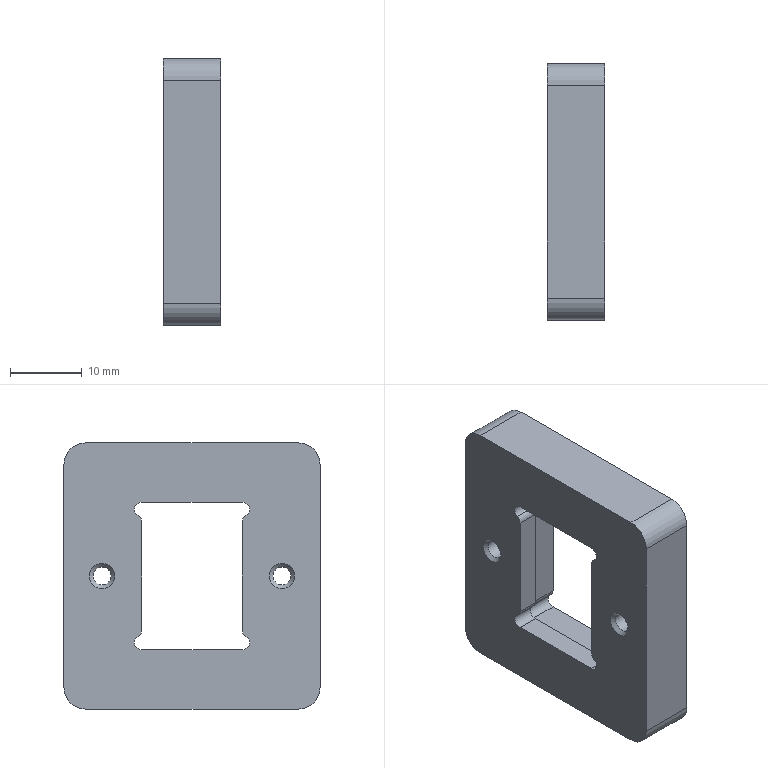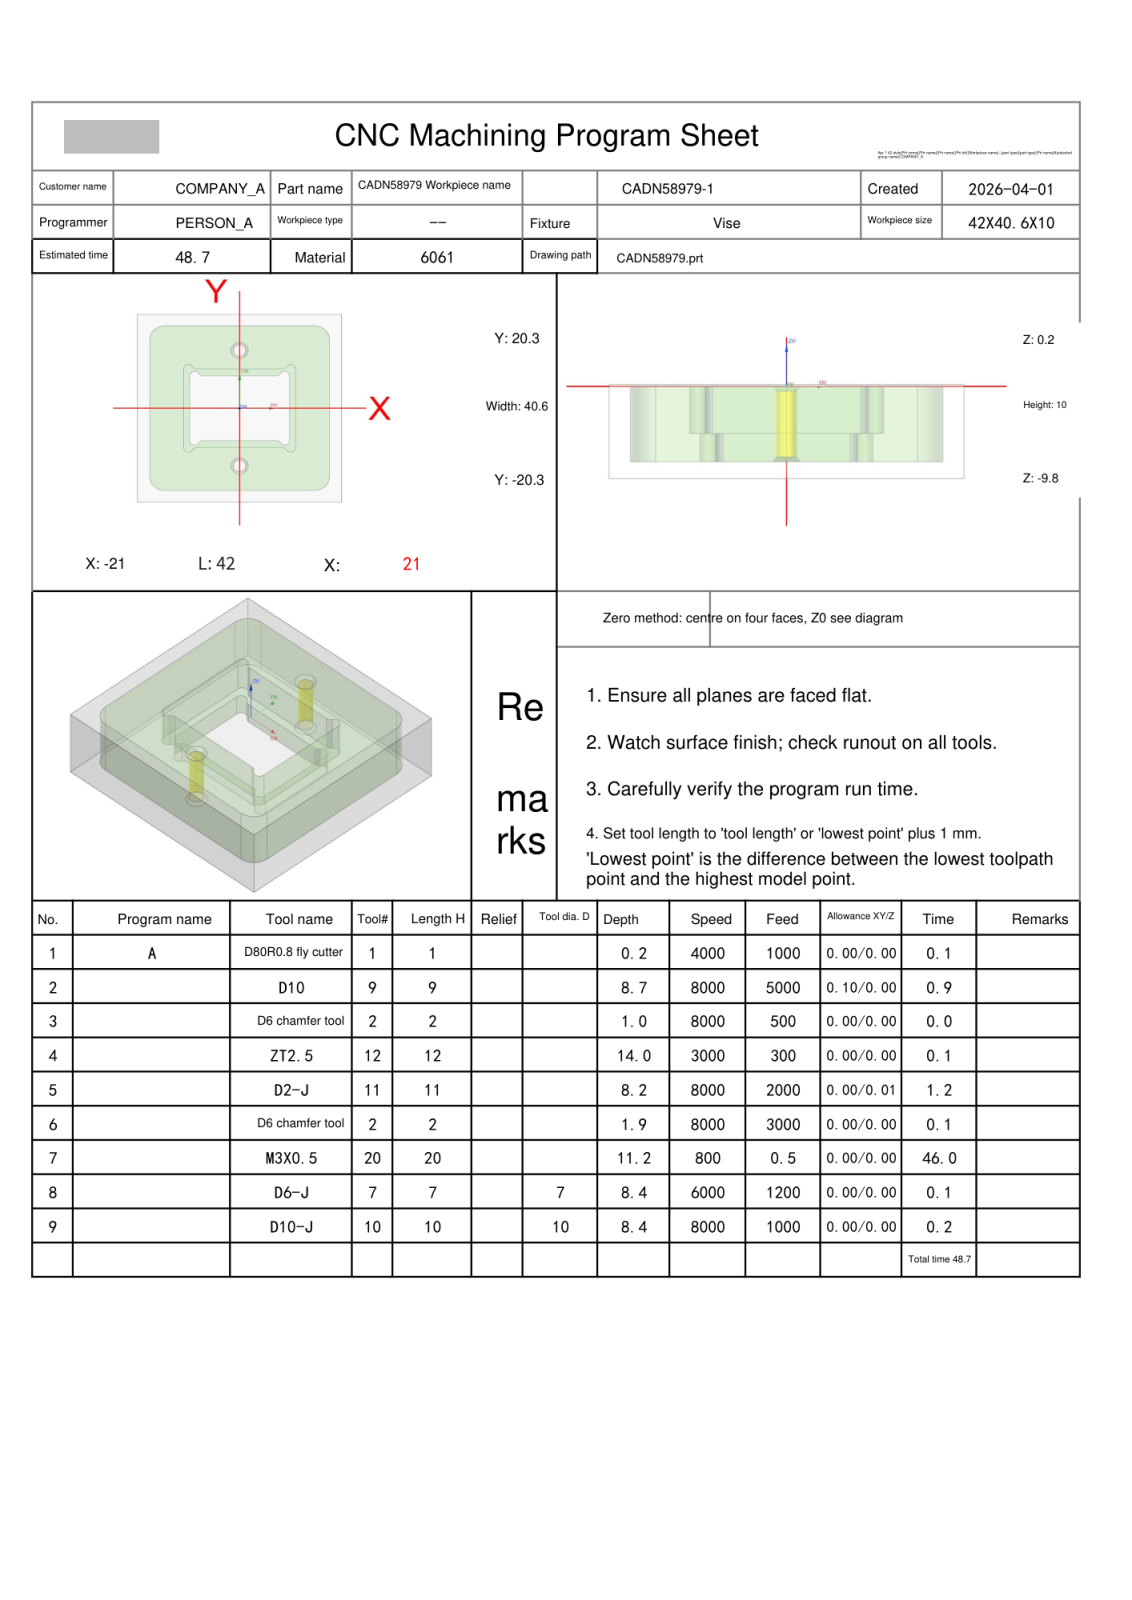NC program | NX | posted by the shop | part box 8 x 35.6 x 37 mm
Lines 315 to 1416 of 3954:
N5 T11 M06
(D2-J  D=2. R=0. H=11 ce=0.00 di=0.01)
G00 G90 G54 X-9.75 Y-2.651 M03 S8000
G43 H11 Z20.
M08
Z.55
G01 X-9.76 Y-2.653 Z.436 F1600.
X-9.786 Y-2.659 Z.333
X-9.828 Y-2.671 Z.242
X-9.882 Y-2.688 Z.161
X-9.944 Y-2.712 Z.089
X-10.014 Y-2.742 Z.027
X-10.088 Y-2.779 Z-.026
X-10.162 Y-2.824 Z-.071
X-10.236 Y-2.877 Z-.109
X-10.306 Y-2.939 Z-.139
X-10.368 Y-3.011 Z-.162
X-10.422 Y-3.092 Z-.179
X-10.464 Y-3.184 Z-.191
X-10.49 Y-3.286 Z-.198
X-10.5 Y-3.401 Z-.2
Y-8.5 F2000.
G02 X-8.768 Y-7.5 I1.732 J-1.
G01 X-6.401
X-6.387 Y-7.484
X-6.398 Y-7.439 Z-.202
X-6.432 Y-7.368 Z-.205
X-6.488 Y-7.273 Z-.209
X-6.707 Y-6.956 Z-.222
X-6.93 Y-6.661 Z-.234
X-7.229 Y-6.288 Z-.25
X-7.746 Y-5.698 Z-.276
X-8.213 Y-5.213 Z-.3
X-8.698 Y-4.746 Z-.323
X-9.288 Y-4.229 Z-.35
X-9.661 Y-3.93 Z-.366
X-9.956 Y-3.707 Z-.378
X-10.273 Y-3.488 Z-.391
X-10.368 Y-3.432 Z-.394
X-10.439 Y-3.398 Z-.397
X-10.484 Y-3.387 Z-.399
X-10.5 Y-3.401 Z-.4
Y-8.5
G02 X-8.768 Y-7.5 I1.732 J-1.
G01 X-6.401
X-6.387 Y-7.484
X-6.398 Y-7.439 Z-.402
X-6.432 Y-7.368 Z-.405
X-6.488 Y-7.273 Z-.409
X-6.707 Y-6.956 Z-.421
X-6.93 Y-6.661 Z-.434
X-7.229 Y-6.288 Z-.45
X-7.746 Y-5.698 Z-.476
X-8.213 Y-5.213 Z-.5
X-8.698 Y-4.746 Z-.523
X-9.288 Y-4.229 Z-.549
X-9.661 Y-3.93 Z-.565
X-9.956 Y-3.707 Z-.578
X-10.273 Y-3.488 Z-.59
X-10.368 Y-3.432 Z-.594
X-10.439 Y-3.398 Z-.597
X-10.484 Y-3.387 Z-.599
X-10.5 Y-3.401
Y-8.5
G02 X-8.768 Y-7.5 I1.732 J-1.
G01 X-6.401
X-6.387 Y-7.484 Z-.6
X-6.398 Y-7.439 Z-.602
X-6.432 Y-7.368 Z-.605
X-6.488 Y-7.273 Z-.608
X-6.707 Y-6.956 Z-.621
X-6.93 Y-6.661 Z-.633
X-7.229 Y-6.288 Z-.649
X-7.746 Y-5.698 Z-.676
X-8.213 Y-5.213 Z-.699
X-8.698 Y-4.746 Z-.723
X-9.288 Y-4.229 Z-.749
X-9.661 Y-3.93 Z-.765
X-9.956 Y-3.707 Z-.777
X-10.273 Y-3.488 Z-.79
X-10.368 Y-3.432 Z-.794
X-10.439 Y-3.398 Z-.797
X-10.484 Y-3.387 Z-.799
X-10.5 Y-3.401
Y-8.5
G02 X-8.768 Y-7.5 I1.732 J-1.
G01 X-6.401
X-6.387 Y-7.484 Z-.8
X-6.398 Y-7.439 Z-.802
X-6.432 Y-7.368 Z-.804
X-6.488 Y-7.273 Z-.808
X-6.707 Y-6.956 Z-.821
X-6.93 Y-6.661 Z-.833
X-7.229 Y-6.288 Z-.849
X-7.746 Y-5.698 Z-.876
X-8.213 Y-5.213 Z-.899
X-8.698 Y-4.746 Z-.922
X-9.288 Y-4.229 Z-.949
X-9.661 Y-3.93 Z-.965
X-9.956 Y-3.707 Z-.977
X-10.273 Y-3.488 Z-.99
X-10.368 Y-3.432 Z-.994
X-10.439 Y-3.398 Z-.997
X-10.484 Y-3.387 Z-.998
X-10.5 Y-3.401 Z-.999
Y-8.5
G02 X-8.768 Y-7.5 I1.732 J-1.
G01 X-6.401
X-6.387 Y-7.484 Z-1.
X-6.398 Y-7.439 Z-1.001
X-6.432 Y-7.368 Z-1.004
X-6.488 Y-7.273 Z-1.008
X-6.707 Y-6.956 Z-1.021
X-6.93 Y-6.661 Z-1.033
X-7.229 Y-6.288 Z-1.049
X-7.746 Y-5.698 Z-1.076
X-8.213 Y-5.213 Z-1.099
X-8.698 Y-4.746 Z-1.122
X-9.288 Y-4.229 Z-1.149
X-9.661 Y-3.93 Z-1.165
X-9.956 Y-3.707 Z-1.177
X-10.273 Y-3.488 Z-1.19
X-10.368 Y-3.432 Z-1.194
X-10.439 Y-3.398 Z-1.196
X-10.484 Y-3.387 Z-1.198
X-10.5 Y-3.401 Z-1.199
Y-8.5
G02 X-8.768 Y-7.5 I1.732 J-1.
G01 X-6.401
X-6.387 Y-7.484
X-6.398 Y-7.439 Z-1.201
X-6.432 Y-7.368 Z-1.204
X-6.488 Y-7.273 Z-1.208
X-6.707 Y-6.956 Z-1.221
X-6.93 Y-6.661 Z-1.233
X-7.229 Y-6.288 Z-1.249
X-7.746 Y-5.698 Z-1.275
X-8.213 Y-5.213 Z-1.299
X-8.698 Y-4.746 Z-1.322
X-9.288 Y-4.229 Z-1.349
X-9.661 Y-3.93 Z-1.365
X-9.956 Y-3.707 Z-1.377
X-10.273 Y-3.488 Z-1.39
X-10.368 Y-3.432 Z-1.393
X-10.439 Y-3.398 Z-1.396
X-10.484 Y-3.387 Z-1.398
X-10.5 Y-3.401 Z-1.399
Y-8.5
G02 X-8.768 Y-7.5 I1.732 J-1.
G01 X-6.401
X-6.387 Y-7.484
X-6.398 Y-7.439 Z-1.401
X-6.432 Y-7.368 Z-1.404
X-6.488 Y-7.273 Z-1.408
X-6.707 Y-6.956 Z-1.42
X-6.93 Y-6.661 Z-1.433
X-7.229 Y-6.288 Z-1.449
X-7.746 Y-5.698 Z-1.475
X-8.213 Y-5.213 Z-1.499
X-8.698 Y-4.746 Z-1.522
X-9.288 Y-4.229 Z-1.548
X-9.661 Y-3.93 Z-1.564
X-9.956 Y-3.707 Z-1.577
X-10.273 Y-3.488 Z-1.589
X-10.368 Y-3.432 Z-1.593
X-10.439 Y-3.398 Z-1.596
X-10.484 Y-3.387 Z-1.598
X-10.5 Y-3.401
Y-8.5
G02 X-8.768 Y-7.5 I1.732 J-1.
G01 X-6.401
X-6.387 Y-7.484 Z-1.599
X-6.398 Y-7.439 Z-1.601
X-6.432 Y-7.368 Z-1.604
X-6.488 Y-7.273 Z-1.607
X-6.707 Y-6.956 Z-1.62
X-6.93 Y-6.661 Z-1.632
X-7.229 Y-6.288 Z-1.648
X-7.746 Y-5.698 Z-1.675
X-8.213 Y-5.213 Z-1.698
X-8.698 Y-4.746 Z-1.722
X-9.288 Y-4.229 Z-1.748
X-9.661 Y-3.93 Z-1.764
X-9.956 Y-3.707 Z-1.776
X-10.273 Y-3.488 Z-1.789
X-10.368 Y-3.432 Z-1.793
X-10.439 Y-3.398 Z-1.796
X-10.484 Y-3.387 Z-1.798
X-10.5 Y-3.401
Y-8.5
G02 X-8.768 Y-7.5 I1.732 J-1.
G01 X-6.401
X-6.387 Y-7.484 Z-1.799
X-6.398 Y-7.439 Z-1.801
X-6.432 Y-7.368 Z-1.803
X-6.488 Y-7.273 Z-1.807
X-6.707 Y-6.956 Z-1.82
X-6.93 Y-6.661 Z-1.832
X-7.229 Y-6.288 Z-1.848
X-7.746 Y-5.698 Z-1.875
X-8.213 Y-5.213 Z-1.898
X-8.698 Y-4.746 Z-1.921
X-9.288 Y-4.229 Z-1.948
X-9.661 Y-3.93 Z-1.964
X-9.956 Y-3.707 Z-1.976
X-10.273 Y-3.488 Z-1.989
X-10.368 Y-3.432 Z-1.993
X-10.439 Y-3.398 Z-1.996
X-10.484 Y-3.387 Z-1.997
X-10.5 Y-3.401 Z-1.998
Y-8.5
G02 X-8.768 Y-7.5 I1.732 J-1.
G01 X-6.401
X-6.387 Y-7.484 Z-1.999
X-6.398 Y-7.439 Z-2.
X-6.432 Y-7.368 Z-2.003
X-6.488 Y-7.273 Z-2.007
X-6.707 Y-6.956 Z-2.02
X-6.93 Y-6.661 Z-2.032
X-7.229 Y-6.288 Z-2.048
X-7.746 Y-5.698 Z-2.075
X-8.213 Y-5.213 Z-2.098
X-8.698 Y-4.746 Z-2.121
X-9.288 Y-4.229 Z-2.148
X-9.661 Y-3.93 Z-2.164
X-9.956 Y-3.707 Z-2.176
X-10.273 Y-3.488 Z-2.189
X-10.368 Y-3.432 Z-2.193
X-10.439 Y-3.398 Z-2.195
X-10.484 Y-3.387 Z-2.197
X-10.5 Y-3.401 Z-2.198
Y-8.5
G02 X-8.768 Y-7.5 I1.732 J-1.
G01 X-6.401
X-6.387 Y-7.484
X-6.398 Y-7.439 Z-2.2
X-6.432 Y-7.368 Z-2.203
X-6.488 Y-7.273 Z-2.207
X-6.707 Y-6.956 Z-2.22
X-6.93 Y-6.661 Z-2.232
X-7.229 Y-6.288 Z-2.248
X-7.746 Y-5.698 Z-2.274
X-8.213 Y-5.213 Z-2.298
X-8.698 Y-4.746 Z-2.321
X-9.288 Y-4.229 Z-2.348
X-9.661 Y-3.93 Z-2.364
X-9.956 Y-3.707 Z-2.376
X-10.273 Y-3.488 Z-2.389
X-10.368 Y-3.432 Z-2.392
X-10.439 Y-3.398 Z-2.395
X-10.484 Y-3.387 Z-2.397
X-10.5 Y-3.401 Z-2.398
Y-8.5
G02 X-8.768 Y-7.5 I1.732 J-1.
G01 X-6.401
X-6.387 Y-7.484
X-6.398 Y-7.439 Z-2.4
X-6.432 Y-7.368 Z-2.403
X-6.488 Y-7.273 Z-2.407
X-6.707 Y-6.956 Z-2.419
X-6.93 Y-6.661 Z-2.432
X-7.229 Y-6.288 Z-2.448
X-7.746 Y-5.698 Z-2.474
X-8.213 Y-5.213 Z-2.498
X-8.698 Y-4.746 Z-2.521
X-9.288 Y-4.229 Z-2.547
X-9.661 Y-3.93 Z-2.563
X-9.956 Y-3.707 Z-2.576
X-10.273 Y-3.488 Z-2.588
X-10.368 Y-3.432 Z-2.592
X-10.439 Y-3.398 Z-2.595
X-10.484 Y-3.387 Z-2.597
X-10.5 Y-3.401
Y-8.5
G02 X-8.768 Y-7.5 I1.732 J-1.
G01 X-6.401
X-6.387 Y-7.484 Z-2.598
X-6.398 Y-7.439 Z-2.6
X-6.432 Y-7.368 Z-2.603
X-6.488 Y-7.273 Z-2.606
X-6.707 Y-6.956 Z-2.619
X-6.93 Y-6.661 Z-2.631
X-7.229 Y-6.288 Z-2.647
X-7.746 Y-5.698 Z-2.674
X-8.213 Y-5.213 Z-2.697
X-8.698 Y-4.746 Z-2.721
X-9.288 Y-4.229 Z-2.747
X-9.661 Y-3.93 Z-2.763
X-9.956 Y-3.707 Z-2.775
X-10.273 Y-3.488 Z-2.788
X-10.368 Y-3.432 Z-2.792
X-10.439 Y-3.398 Z-2.795
X-10.484 Y-3.387 Z-2.797
X-10.5 Y-3.401
Y-8.5
G02 X-8.768 Y-7.5 I1.732 J-1.
G01 X-6.401
X-6.387 Y-7.484 Z-2.798
X-6.398 Y-7.439 Z-2.8
X-6.432 Y-7.368 Z-2.802
X-6.488 Y-7.273 Z-2.806
X-6.707 Y-6.956 Z-2.819
X-6.93 Y-6.661 Z-2.831
X-7.229 Y-6.288 Z-2.847
X-7.746 Y-5.698 Z-2.874
X-8.213 Y-5.213 Z-2.897
X-8.698 Y-4.746 Z-2.92
X-9.288 Y-4.229 Z-2.947
X-9.661 Y-3.93 Z-2.963
X-9.956 Y-3.707 Z-2.975
X-10.273 Y-3.488 Z-2.988
X-10.368 Y-3.432 Z-2.992
X-10.439 Y-3.398 Z-2.995
X-10.484 Y-3.387 Z-2.996
X-10.5 Y-3.401 Z-2.997
Y-8.5
G02 X-8.768 Y-7.5 I1.732 J-1.
G01 X-6.401
X-6.387 Y-7.484 Z-2.998
X-6.398 Y-7.439 Z-2.999
X-6.432 Y-7.368 Z-3.002
X-6.488 Y-7.273 Z-3.006
X-6.707 Y-6.956 Z-3.019
X-6.93 Y-6.661 Z-3.031
X-7.229 Y-6.288 Z-3.047
X-7.746 Y-5.698 Z-3.074
X-8.213 Y-5.213 Z-3.097
X-8.698 Y-4.746 Z-3.12
X-9.288 Y-4.229 Z-3.147
X-9.661 Y-3.93 Z-3.163
X-9.956 Y-3.707 Z-3.175
X-10.273 Y-3.488 Z-3.188
X-10.368 Y-3.432 Z-3.192
X-10.439 Y-3.398 Z-3.194
X-10.484 Y-3.387 Z-3.196
X-10.5 Y-3.401 Z-3.197
Y-8.5
G02 X-8.768 Y-7.5 I1.732 J-1.
G01 X-6.401
X-6.387 Y-7.484
X-6.398 Y-7.439 Z-3.199
X-6.432 Y-7.368 Z-3.202
X-6.488 Y-7.273 Z-3.206
X-6.707 Y-6.956 Z-3.219
X-6.93 Y-6.661 Z-3.231
X-7.229 Y-6.288 Z-3.247
X-7.746 Y-5.698 Z-3.273
X-8.213 Y-5.213 Z-3.297
X-8.698 Y-4.746 Z-3.32
X-9.288 Y-4.229 Z-3.347
X-9.661 Y-3.93 Z-3.363
X-9.956 Y-3.707 Z-3.375
X-10.273 Y-3.488 Z-3.388
X-10.368 Y-3.432 Z-3.391
X-10.439 Y-3.398 Z-3.394
X-10.484 Y-3.387 Z-3.396
X-10.5 Y-3.401 Z-3.397
Y-8.5
G02 X-8.768 Y-7.5 I1.732 J-1.
G01 X-6.401
X-6.387 Y-7.484
X-6.398 Y-7.439 Z-3.399
X-6.432 Y-7.368 Z-3.402
X-6.488 Y-7.273 Z-3.406
X-6.707 Y-6.956 Z-3.418
X-6.93 Y-6.661 Z-3.431
X-7.229 Y-6.288 Z-3.447
X-7.746 Y-5.698 Z-3.473
X-8.213 Y-5.213 Z-3.497
X-8.698 Y-4.746 Z-3.52
X-9.288 Y-4.229 Z-3.546
X-9.661 Y-3.93 Z-3.562
X-9.956 Y-3.707 Z-3.575
X-10.273 Y-3.488 Z-3.587
X-10.368 Y-3.432 Z-3.591
X-10.439 Y-3.398 Z-3.594
X-10.484 Y-3.387 Z-3.596
X-10.5 Y-3.401
Y-8.5
G02 X-8.768 Y-7.5 I1.732 J-1.
G01 X-6.401
X-6.387 Y-7.484 Z-3.597
X-6.398 Y-7.439 Z-3.599
X-6.432 Y-7.368 Z-3.602
X-6.488 Y-7.273 Z-3.605
X-6.707 Y-6.956 Z-3.618
X-6.93 Y-6.661 Z-3.63
X-7.229 Y-6.288 Z-3.646
X-7.746 Y-5.698 Z-3.673
X-8.213 Y-5.213 Z-3.696
X-8.698 Y-4.746 Z-3.72
X-9.288 Y-4.229 Z-3.746
X-9.661 Y-3.93 Z-3.762
X-9.956 Y-3.707 Z-3.774
X-10.273 Y-3.488 Z-3.787
X-10.368 Y-3.432 Z-3.791
X-10.439 Y-3.398 Z-3.794
X-10.484 Y-3.387 Z-3.796
X-10.5 Y-3.401
Y-8.5
G02 X-8.768 Y-7.5 I1.732 J-1.
G01 X-6.401
X-6.387 Y-7.484 Z-3.797
X-6.398 Y-7.439 Z-3.799
X-6.432 Y-7.368 Z-3.801
X-6.488 Y-7.273 Z-3.805
X-6.707 Y-6.956 Z-3.818
X-6.93 Y-6.661 Z-3.83
X-7.229 Y-6.288 Z-3.846
X-7.746 Y-5.698 Z-3.873
X-8.213 Y-5.213 Z-3.896
X-8.698 Y-4.746 Z-3.919
X-9.288 Y-4.229 Z-3.946
X-9.661 Y-3.93 Z-3.962
X-9.956 Y-3.707 Z-3.974
X-10.273 Y-3.488 Z-3.987
X-10.368 Y-3.432 Z-3.991
X-10.439 Y-3.398 Z-3.994
X-10.484 Y-3.387 Z-3.995
X-10.5 Y-3.401 Z-3.996
Y-8.5
G02 X-8.768 Y-7.5 I1.732 J-1.
G01 X-6.401
X-6.387 Y-7.484 Z-3.997
X-6.398 Y-7.439 Z-3.998
X-6.432 Y-7.368 Z-4.001
X-6.488 Y-7.273 Z-4.005
X-6.707 Y-6.956 Z-4.018
X-6.93 Y-6.661 Z-4.03
X-7.229 Y-6.288 Z-4.046
X-7.746 Y-5.698 Z-4.073
X-8.213 Y-5.213 Z-4.096
X-8.698 Y-4.746 Z-4.119
X-9.288 Y-4.229 Z-4.146
X-9.661 Y-3.93 Z-4.162
X-9.956 Y-3.707 Z-4.174
X-10.273 Y-3.488 Z-4.187
X-10.368 Y-3.432 Z-4.191
X-10.439 Y-3.398 Z-4.193
X-10.484 Y-3.387 Z-4.195
X-10.5 Y-3.401 Z-4.196
Y-8.5
G02 X-8.768 Y-7.5 I1.732 J-1.
G01 X-6.401
X-6.387 Y-7.484
X-6.398 Y-7.439 Z-4.198
X-6.432 Y-7.368 Z-4.201
X-6.488 Y-7.273 Z-4.205
X-6.707 Y-6.956 Z-4.218
X-6.93 Y-6.661 Z-4.23
X-7.229 Y-6.288 Z-4.246
X-7.746 Y-5.698 Z-4.272
X-8.213 Y-5.213 Z-4.296
X-8.698 Y-4.746 Z-4.319
X-9.288 Y-4.229 Z-4.346
X-9.661 Y-3.93 Z-4.362
X-9.956 Y-3.707 Z-4.374
X-10.273 Y-3.488 Z-4.387
X-10.368 Y-3.432 Z-4.39
X-10.439 Y-3.398 Z-4.393
X-10.484 Y-3.387 Z-4.395
X-10.5 Y-3.401 Z-4.396
Y-8.5
G02 X-8.768 Y-7.5 I1.732 J-1.
G01 X-6.401
X-6.387 Y-7.484
X-6.398 Y-7.439 Z-4.398
X-6.432 Y-7.368 Z-4.401
X-6.488 Y-7.273 Z-4.405
X-6.707 Y-6.956 Z-4.417
X-6.93 Y-6.661 Z-4.43
X-7.229 Y-6.288 Z-4.446
X-7.746 Y-5.698 Z-4.472
X-8.213 Y-5.213 Z-4.496
X-8.698 Y-4.746 Z-4.519
X-9.288 Y-4.229 Z-4.545
X-9.661 Y-3.93 Z-4.561
X-9.956 Y-3.707 Z-4.574
X-10.273 Y-3.488 Z-4.586
X-10.368 Y-3.432 Z-4.59
X-10.439 Y-3.398 Z-4.593
X-10.484 Y-3.387 Z-4.595
X-10.5 Y-3.401
Y-8.5
G02 X-8.768 Y-7.5 I1.732 J-1.
G01 X-6.401
X-6.387 Y-7.484 Z-4.596
X-6.398 Y-7.439 Z-4.598
X-6.432 Y-7.368 Z-4.601
X-6.488 Y-7.273 Z-4.604
X-6.707 Y-6.956 Z-4.617
X-6.93 Y-6.661 Z-4.629
X-7.229 Y-6.288 Z-4.645
X-7.746 Y-5.698 Z-4.672
X-8.213 Y-5.213 Z-4.695
X-8.698 Y-4.746 Z-4.719
X-9.288 Y-4.229 Z-4.745
X-9.661 Y-3.93 Z-4.761
X-9.956 Y-3.707 Z-4.773
X-10.273 Y-3.488 Z-4.786
X-10.368 Y-3.432 Z-4.79
X-10.439 Y-3.398 Z-4.793
X-10.484 Y-3.387 Z-4.795
X-10.5 Y-3.401
Y-8.5
G02 X-8.768 Y-7.5 I1.732 J-1.
G01 X-6.401
X-6.387 Y-7.484 Z-4.796
X-6.398 Y-7.439 Z-4.798
X-6.432 Y-7.368 Z-4.8
X-6.488 Y-7.273 Z-4.804
X-6.707 Y-6.956 Z-4.817
X-6.93 Y-6.661 Z-4.829
X-7.229 Y-6.288 Z-4.845
X-7.746 Y-5.698 Z-4.872
X-8.213 Y-5.213 Z-4.895
X-8.698 Y-4.746 Z-4.918
X-9.288 Y-4.229 Z-4.945
X-9.661 Y-3.93 Z-4.961
X-9.956 Y-3.707 Z-4.973
X-10.273 Y-3.488 Z-4.986
X-10.368 Y-3.432 Z-4.99
X-10.439 Y-3.398 Z-4.993
X-10.484 Y-3.387 Z-4.994
X-10.5 Y-3.401 Z-4.995
Y-8.5
G02 X-8.768 Y-7.5 I1.732 J-1.
G01 X-6.401
X-6.286 Y-7.49 Z-4.993
X-6.184 Y-7.464 Z-4.986
X-6.092 Y-7.422 Z-4.975
X-6.011 Y-7.368 Z-4.957
X-5.939 Y-7.306 Z-4.934
X-5.877 Y-7.236 Z-4.904
X-5.824 Y-7.162 Z-4.867
X-5.779 Y-7.088 Z-4.821
X-5.742 Y-7.014 Z-4.768
X-5.712 Y-6.944 Z-4.706
X-5.688 Y-6.882 Z-4.635
X-5.671 Y-6.828 Z-4.553
X-5.659 Y-6.786 Z-4.462
X-5.653 Y-6.76 Z-4.359
X-5.651 Y-6.75 Z-4.245
G00 Z3.
X5.651
Z.55
G01 X5.653 Y-6.76 Z.436 F1600.
X5.659 Y-6.786 Z.333
X5.671 Y-6.828 Z.242
X5.688 Y-6.882 Z.161
X5.712 Y-6.944 Z.089
X5.742 Y-7.014 Z.027
X5.779 Y-7.088 Z-.026
X5.824 Y-7.162 Z-.071
X5.877 Y-7.236 Z-.109
X5.939 Y-7.306 Z-.139
X6.011 Y-7.368 Z-.162
X6.092 Y-7.422 Z-.179
X6.184 Y-7.464 Z-.191
X6.286 Y-7.49 Z-.198
X6.401 Y-7.5 Z-.2
X8.768 F2000.
G02 X10.5 Y-8.5 I0.0 J-2.
G01 Y-3.401
X10.484 Y-3.387
X10.439 Y-3.398 Z-.202
X10.368 Y-3.432 Z-.205
X10.273 Y-3.488 Z-.209
X9.956 Y-3.707 Z-.222
X9.661 Y-3.93 Z-.234
X9.288 Y-4.229 Z-.25
X8.698 Y-4.746 Z-.276
X8.213 Y-5.213 Z-.3
X7.746 Y-5.698 Z-.323
X7.229 Y-6.288 Z-.35
X6.93 Y-6.661 Z-.366
X6.707 Y-6.956 Z-.378
X6.488 Y-7.273 Z-.391
X6.432 Y-7.368 Z-.394
X6.398 Y-7.439 Z-.397
X6.387 Y-7.484 Z-.399
X6.401 Y-7.5 Z-.4
X8.768
G02 X10.5 Y-8.5 I0.0 J-2.
G01 Y-3.401
X10.484 Y-3.387
X10.439 Y-3.398 Z-.402
X10.368 Y-3.432 Z-.405
X10.273 Y-3.488 Z-.409
X9.956 Y-3.707 Z-.421
X9.661 Y-3.93 Z-.434
X9.288 Y-4.229 Z-.45
X8.698 Y-4.746 Z-.476
X8.213 Y-5.213 Z-.5
X7.746 Y-5.698 Z-.523
X7.229 Y-6.288 Z-.549
X6.93 Y-6.661 Z-.565
X6.707 Y-6.956 Z-.578
X6.488 Y-7.273 Z-.59
X6.432 Y-7.368 Z-.594
X6.398 Y-7.439 Z-.597
X6.387 Y-7.484 Z-.599
X6.401 Y-7.5
X8.768
G02 X10.5 Y-8.5 I0.0 J-2.
G01 Y-3.401
X10.484 Y-3.387 Z-.6
X10.439 Y-3.398 Z-.602
X10.368 Y-3.432 Z-.605
X10.273 Y-3.488 Z-.608
X9.956 Y-3.707 Z-.621
X9.661 Y-3.93 Z-.633
X9.288 Y-4.229 Z-.649
X8.698 Y-4.746 Z-.676
X8.213 Y-5.213 Z-.699
X7.746 Y-5.698 Z-.723
X7.229 Y-6.288 Z-.749
X6.93 Y-6.661 Z-.765
X6.707 Y-6.956 Z-.777
X6.488 Y-7.273 Z-.79
X6.432 Y-7.368 Z-.794
X6.398 Y-7.439 Z-.797
X6.387 Y-7.484 Z-.799
X6.401 Y-7.5
X8.768
G02 X10.5 Y-8.5 I0.0 J-2.
G01 Y-3.401
X10.484 Y-3.387 Z-.8
X10.439 Y-3.398 Z-.802
X10.368 Y-3.432 Z-.804
X10.273 Y-3.488 Z-.808
X9.956 Y-3.707 Z-.821
X9.661 Y-3.93 Z-.833
X9.288 Y-4.229 Z-.849
X8.698 Y-4.746 Z-.876
X8.213 Y-5.213 Z-.899
X7.746 Y-5.698 Z-.922
X7.229 Y-6.288 Z-.949
X6.93 Y-6.661 Z-.965
X6.707 Y-6.956 Z-.977
X6.488 Y-7.273 Z-.99
X6.432 Y-7.368 Z-.994
X6.398 Y-7.439 Z-.997
X6.387 Y-7.484 Z-.998
X6.401 Y-7.5 Z-.999
X8.768
G02 X10.5 Y-8.5 I0.0 J-2.
G01 Y-3.401
X10.484 Y-3.387 Z-1.
X10.439 Y-3.398 Z-1.001
X10.368 Y-3.432 Z-1.004
X10.273 Y-3.488 Z-1.008
X9.956 Y-3.707 Z-1.021
X9.661 Y-3.93 Z-1.033
X9.288 Y-4.229 Z-1.049
X8.698 Y-4.746 Z-1.076
X8.213 Y-5.213 Z-1.099
X7.746 Y-5.698 Z-1.122
X7.229 Y-6.288 Z-1.149
X6.93 Y-6.661 Z-1.165
X6.707 Y-6.956 Z-1.177
X6.488 Y-7.273 Z-1.19
X6.432 Y-7.368 Z-1.194
X6.398 Y-7.439 Z-1.196
X6.387 Y-7.484 Z-1.198
X6.401 Y-7.5 Z-1.199
X8.768
G02 X10.5 Y-8.5 I0.0 J-2.
G01 Y-3.401
X10.484 Y-3.387
X10.439 Y-3.398 Z-1.201
X10.368 Y-3.432 Z-1.204
X10.273 Y-3.488 Z-1.208
X9.956 Y-3.707 Z-1.221
X9.661 Y-3.93 Z-1.233
X9.288 Y-4.229 Z-1.249
X8.698 Y-4.746 Z-1.275
X8.213 Y-5.213 Z-1.299
X7.746 Y-5.698 Z-1.322
X7.229 Y-6.288 Z-1.349
X6.93 Y-6.661 Z-1.365
X6.707 Y-6.956 Z-1.377
X6.488 Y-7.273 Z-1.39
X6.432 Y-7.368 Z-1.393
X6.398 Y-7.439 Z-1.396
X6.387 Y-7.484 Z-1.398
X6.401 Y-7.5 Z-1.399
X8.768
G02 X10.5 Y-8.5 I0.0 J-2.
G01 Y-3.401
X10.484 Y-3.387
X10.439 Y-3.398 Z-1.401
X10.368 Y-3.432 Z-1.404
X10.273 Y-3.488 Z-1.408
X9.956 Y-3.707 Z-1.42
X9.661 Y-3.93 Z-1.433
X9.288 Y-4.229 Z-1.449
X8.698 Y-4.746 Z-1.475
X8.213 Y-5.213 Z-1.499
X7.746 Y-5.698 Z-1.522
X7.229 Y-6.288 Z-1.548
X6.93 Y-6.661 Z-1.564
X6.707 Y-6.956 Z-1.577
X6.488 Y-7.273 Z-1.589
X6.432 Y-7.368 Z-1.593
X6.398 Y-7.439 Z-1.596
X6.387 Y-7.484 Z-1.598
X6.401 Y-7.5
X8.768
G02 X10.5 Y-8.5 I0.0 J-2.
G01 Y-3.401
X10.484 Y-3.387 Z-1.599
X10.439 Y-3.398 Z-1.601
X10.368 Y-3.432 Z-1.604
X10.273 Y-3.488 Z-1.607
X9.956 Y-3.707 Z-1.62
X9.661 Y-3.93 Z-1.632
X9.288 Y-4.229 Z-1.648
X8.698 Y-4.746 Z-1.675
X8.213 Y-5.213 Z-1.698
X7.746 Y-5.698 Z-1.722
X7.229 Y-6.288 Z-1.748
X6.93 Y-6.661 Z-1.764
X6.707 Y-6.956 Z-1.776
X6.488 Y-7.273 Z-1.789
X6.432 Y-7.368 Z-1.793
X6.398 Y-7.439 Z-1.796
X6.387 Y-7.484 Z-1.798
X6.401 Y-7.5
X8.768
G02 X10.5 Y-8.5 I0.0 J-2.
G01 Y-3.401
X10.484 Y-3.387 Z-1.799
X10.439 Y-3.398 Z-1.801
X10.368 Y-3.432 Z-1.803
X10.273 Y-3.488 Z-1.807
X9.956 Y-3.707 Z-1.82
X9.661 Y-3.93 Z-1.832
X9.288 Y-4.229 Z-1.848
X8.698 Y-4.746 Z-1.875
X8.213 Y-5.213 Z-1.898
X7.746 Y-5.698 Z-1.921
X7.229 Y-6.288 Z-1.948
X6.93 Y-6.661 Z-1.964
X6.707 Y-6.956 Z-1.976
X6.488 Y-7.273 Z-1.989
X6.432 Y-7.368 Z-1.993
X6.398 Y-7.439 Z-1.996
X6.387 Y-7.484 Z-1.997
X6.401 Y-7.5 Z-1.998
X8.768
G02 X10.5 Y-8.5 I0.0 J-2.
G01 Y-3.401
X10.484 Y-3.387 Z-1.999
X10.439 Y-3.398 Z-2.
X10.368 Y-3.432 Z-2.003
X10.273 Y-3.488 Z-2.007
X9.956 Y-3.707 Z-2.02
X9.661 Y-3.93 Z-2.032
X9.288 Y-4.229 Z-2.048
X8.698 Y-4.746 Z-2.075
X8.213 Y-5.213 Z-2.098
X7.746 Y-5.698 Z-2.121
X7.229 Y-6.288 Z-2.148
X6.93 Y-6.661 Z-2.164
X6.707 Y-6.956 Z-2.176
X6.488 Y-7.273 Z-2.189
X6.432 Y-7.368 Z-2.193
X6.398 Y-7.439 Z-2.195
X6.387 Y-7.484 Z-2.197
X6.401 Y-7.5 Z-2.198
X8.768
G02 X10.5 Y-8.5 I0.0 J-2.
G01 Y-3.401
X10.484 Y-3.387
X10.439 Y-3.398 Z-2.2
X10.368 Y-3.432 Z-2.203
X10.273 Y-3.488 Z-2.207
X9.956 Y-3.707 Z-2.22
X9.661 Y-3.93 Z-2.232
X9.288 Y-4.229 Z-2.248
X8.698 Y-4.746 Z-2.274
X8.213 Y-5.213 Z-2.298
X7.746 Y-5.698 Z-2.321
X7.229 Y-6.288 Z-2.348
X6.93 Y-6.661 Z-2.364
X6.707 Y-6.956 Z-2.376
X6.488 Y-7.273 Z-2.389
X6.432 Y-7.368 Z-2.392
X6.398 Y-7.439 Z-2.395
X6.387 Y-7.484 Z-2.397
X6.401 Y-7.5 Z-2.398
X8.768
G02 X10.5 Y-8.5 I0.0 J-2.
G01 Y-3.401
X10.484 Y-3.387
X10.439 Y-3.398 Z-2.4
X10.368 Y-3.432 Z-2.403
X10.273 Y-3.488 Z-2.407
X9.956 Y-3.707 Z-2.419
X9.661 Y-3.93 Z-2.432
X9.288 Y-4.229 Z-2.448
X8.698 Y-4.746 Z-2.474
X8.213 Y-5.213 Z-2.498
X7.746 Y-5.698 Z-2.521
X7.229 Y-6.288 Z-2.547
X6.93 Y-6.661 Z-2.563
X6.707 Y-6.956 Z-2.576
X6.488 Y-7.273 Z-2.588
X6.432 Y-7.368 Z-2.592
X6.398 Y-7.439 Z-2.595
X6.387 Y-7.484 Z-2.597
X6.401 Y-7.5
X8.768
G02 X10.5 Y-8.5 I0.0 J-2.
G01 Y-3.401
X10.484 Y-3.387 Z-2.598
X10.439 Y-3.398 Z-2.6
X10.368 Y-3.432 Z-2.603
X10.273 Y-3.488 Z-2.606
X9.956 Y-3.707 Z-2.619
X9.661 Y-3.93 Z-2.631
X9.288 Y-4.229 Z-2.647
X8.698 Y-4.746 Z-2.674
X8.213 Y-5.213 Z-2.697
X7.746 Y-5.698 Z-2.721
X7.229 Y-6.288 Z-2.747
X6.93 Y-6.661 Z-2.763
X6.707 Y-6.956 Z-2.775
X6.488 Y-7.273 Z-2.788
X6.432 Y-7.368 Z-2.792
X6.398 Y-7.439 Z-2.795
X6.387 Y-7.484 Z-2.797
X6.401 Y-7.5
X8.768
G02 X10.5 Y-8.5 I0.0 J-2.
G01 Y-3.401
X10.484 Y-3.387 Z-2.798
X10.439 Y-3.398 Z-2.8
X10.368 Y-3.432 Z-2.802
X10.273 Y-3.488 Z-2.806
X9.956 Y-3.707 Z-2.819
X9.661 Y-3.93 Z-2.831
X9.288 Y-4.229 Z-2.847
X8.698 Y-4.746 Z-2.874
X8.213 Y-5.213 Z-2.897
X7.746 Y-5.698 Z-2.92
X7.229 Y-6.288 Z-2.947
X6.93 Y-6.661 Z-2.963
X6.707 Y-6.956 Z-2.975
X6.488 Y-7.273 Z-2.988
X6.432 Y-7.368 Z-2.992
X6.398 Y-7.439 Z-2.995
X6.387 Y-7.484 Z-2.996
X6.401 Y-7.5 Z-2.997
X8.768
G02 X10.5 Y-8.5 I0.0 J-2.
G01 Y-3.401
X10.484 Y-3.387 Z-2.998
X10.439 Y-3.398 Z-2.999
X10.368 Y-3.432 Z-3.002
X10.273 Y-3.488 Z-3.006
X9.956 Y-3.707 Z-3.019
X9.661 Y-3.93 Z-3.031
X9.288 Y-4.229 Z-3.047
X8.698 Y-4.746 Z-3.074
X8.213 Y-5.213 Z-3.097
X7.746 Y-5.698 Z-3.12
X7.229 Y-6.288 Z-3.147
X6.93 Y-6.661 Z-3.163
X6.707 Y-6.956 Z-3.175
X6.488 Y-7.273 Z-3.188
X6.432 Y-7.368 Z-3.192
X6.398 Y-7.439 Z-3.194
X6.387 Y-7.484 Z-3.196
X6.401 Y-7.5 Z-3.197
X8.768
G02 X10.5 Y-8.5 I0.0 J-2.
G01 Y-3.401
X10.484 Y-3.387
X10.439 Y-3.398 Z-3.199
X10.368 Y-3.432 Z-3.202
X10.273 Y-3.488 Z-3.206
X9.956 Y-3.707 Z-3.219
X9.661 Y-3.93 Z-3.231
X9.288 Y-4.229 Z-3.247
X8.698 Y-4.746 Z-3.273
X8.213 Y-5.213 Z-3.297
X7.746 Y-5.698 Z-3.32
X7.229 Y-6.288 Z-3.347
X6.93 Y-6.661 Z-3.363
X6.707 Y-6.956 Z-3.375
X6.488 Y-7.273 Z-3.388
X6.432 Y-7.368 Z-3.391
X6.398 Y-7.439 Z-3.394
X6.387 Y-7.484 Z-3.396
X6.401 Y-7.5 Z-3.397
X8.768
G02 X10.5 Y-8.5 I0.0 J-2.
G01 Y-3.401
X10.484 Y-3.387
X10.439 Y-3.398 Z-3.399
X10.368 Y-3.432 Z-3.402
X10.273 Y-3.488 Z-3.406
X9.956 Y-3.707 Z-3.418
X9.661 Y-3.93 Z-3.431
X9.288 Y-4.229 Z-3.447
X8.698 Y-4.746 Z-3.473
X8.213 Y-5.213 Z-3.497
X7.746 Y-5.698 Z-3.52
X7.229 Y-6.288 Z-3.546
X6.93 Y-6.661 Z-3.562
X6.707 Y-6.956 Z-3.575
X6.488 Y-7.273 Z-3.587
X6.432 Y-7.368 Z-3.591
X6.398 Y-7.439 Z-3.594
X6.387 Y-7.484 Z-3.596
X6.401 Y-7.5
X8.768
G02 X10.5 Y-8.5 I0.0 J-2.
G01 Y-3.401
X10.484 Y-3.387 Z-3.597
X10.439 Y-3.398 Z-3.599
X10.368 Y-3.432 Z-3.602
X10.273 Y-3.488 Z-3.605
X9.956 Y-3.707 Z-3.618
X9.661 Y-3.93 Z-3.63
X9.288 Y-4.229 Z-3.646
X8.698 Y-4.746 Z-3.673
X8.213 Y-5.213 Z-3.696
X7.746 Y-5.698 Z-3.72
X7.229 Y-6.288 Z-3.746
X6.93 Y-6.661 Z-3.762
X6.707 Y-6.956 Z-3.774
X6.488 Y-7.273 Z-3.787
X6.432 Y-7.368 Z-3.791
X6.398 Y-7.439 Z-3.794
X6.387 Y-7.484 Z-3.796
X6.401 Y-7.5
X8.768
G02 X10.5 Y-8.5 I0.0 J-2.
G01 Y-3.401
X10.484 Y-3.387 Z-3.797
X10.439 Y-3.398 Z-3.799
X10.368 Y-3.432 Z-3.801
X10.273 Y-3.488 Z-3.805
X9.956 Y-3.707 Z-3.818
X9.661 Y-3.93 Z-3.83
X9.288 Y-4.229 Z-3.846
X8.698 Y-4.746 Z-3.873
X8.213 Y-5.213 Z-3.896
X7.746 Y-5.698 Z-3.919
X7.229 Y-6.288 Z-3.946
X6.93 Y-6.661 Z-3.962
X6.707 Y-6.956 Z-3.974
X6.488 Y-7.273 Z-3.987
X6.432 Y-7.368 Z-3.991
X6.398 Y-7.439 Z-3.994
X6.387 Y-7.484 Z-3.995
X6.401 Y-7.5 Z-3.996
X8.768
G02 X10.5 Y-8.5 I0.0 J-2.
G01 Y-3.401
X10.484 Y-3.387 Z-3.997
X10.439 Y-3.398 Z-3.998
X10.368 Y-3.432 Z-4.001
X10.273 Y-3.488 Z-4.005
X9.956 Y-3.707 Z-4.018
X9.661 Y-3.93 Z-4.03
X9.288 Y-4.229 Z-4.046
X8.698 Y-4.746 Z-4.073
X8.213 Y-5.213 Z-4.096
X7.746 Y-5.698 Z-4.119
X7.229 Y-6.288 Z-4.146
X6.93 Y-6.661 Z-4.162
X6.707 Y-6.956 Z-4.174
X6.488 Y-7.273 Z-4.187
X6.432 Y-7.368 Z-4.191
X6.398 Y-7.439 Z-4.193
X6.387 Y-7.484 Z-4.195
X6.401 Y-7.5 Z-4.196
X8.768
G02 X10.5 Y-8.5 I0.0 J-2.
G01 Y-3.401
X10.484 Y-3.387
X10.439 Y-3.398 Z-4.198
X10.368 Y-3.432 Z-4.201
X10.273 Y-3.488 Z-4.205
X9.956 Y-3.707 Z-4.218
X9.661 Y-3.93 Z-4.23
X9.288 Y-4.229 Z-4.246
X8.698 Y-4.746 Z-4.272
X8.213 Y-5.213 Z-4.296
X7.746 Y-5.698 Z-4.319
X7.229 Y-6.288 Z-4.346
X6.93 Y-6.661 Z-4.362
X6.707 Y-6.956 Z-4.374
X6.488 Y-7.273 Z-4.387
X6.432 Y-7.368 Z-4.39
X6.398 Y-7.439 Z-4.393
X6.387 Y-7.484 Z-4.395
X6.401 Y-7.5 Z-4.396
X8.768
G02 X10.5 Y-8.5 I0.0 J-2.
G01 Y-3.401
X10.484 Y-3.387
X10.439 Y-3.398 Z-4.398
X10.368 Y-3.432 Z-4.401
X10.273 Y-3.488 Z-4.405
X9.956 Y-3.707 Z-4.417
X9.661 Y-3.93 Z-4.43
X9.288 Y-4.229 Z-4.446
X8.698 Y-4.746 Z-4.472
X8.213 Y-5.213 Z-4.496
X7.746 Y-5.698 Z-4.519
X7.229 Y-6.288 Z-4.545
X6.93 Y-6.661 Z-4.561
X6.707 Y-6.956 Z-4.574
X6.488 Y-7.273 Z-4.586
X6.432 Y-7.368 Z-4.59
X6.398 Y-7.439 Z-4.593
X6.387 Y-7.484 Z-4.595
X6.401 Y-7.5
X8.768
G02 X10.5 Y-8.5 I0.0 J-2.
G01 Y-3.401
X10.484 Y-3.387 Z-4.596
X10.439 Y-3.398 Z-4.598
X10.368 Y-3.432 Z-4.601
X10.273 Y-3.488 Z-4.604
X9.956 Y-3.707 Z-4.617
X9.661 Y-3.93 Z-4.629
X9.288 Y-4.229 Z-4.645
X8.698 Y-4.746 Z-4.672
X8.213 Y-5.213 Z-4.695
X7.746 Y-5.698 Z-4.719
X7.229 Y-6.288 Z-4.745
X6.93 Y-6.661 Z-4.761
X6.707 Y-6.956 Z-4.773
X6.488 Y-7.273 Z-4.786
X6.432 Y-7.368 Z-4.79
X6.398 Y-7.439 Z-4.793
X6.387 Y-7.484 Z-4.795
X6.401 Y-7.5
X8.768
G02 X10.5 Y-8.5 I0.0 J-2.
G01 Y-3.401
X10.484 Y-3.387 Z-4.796
X10.439 Y-3.398 Z-4.798
X10.368 Y-3.432 Z-4.8
X10.273 Y-3.488 Z-4.804
X9.956 Y-3.707 Z-4.817
X9.661 Y-3.93 Z-4.829
X9.288 Y-4.229 Z-4.845
X8.698 Y-4.746 Z-4.872
X8.213 Y-5.213 Z-4.895
X7.746 Y-5.698 Z-4.918
X7.229 Y-6.288 Z-4.945
X6.93 Y-6.661 Z-4.961
X6.707 Y-6.956 Z-4.973
X6.488 Y-7.273 Z-4.986
X6.432 Y-7.368 Z-4.99
X6.398 Y-7.439 Z-4.993
X6.387 Y-7.484 Z-4.994
X6.401 Y-7.5 Z-4.995
X8.768
G02 X10.5 Y-8.5 I0.0 J-2.
G01 Y-3.401
X10.49 Y-3.286 Z-4.993
X10.464 Y-3.184 Z-4.986
X10.422 Y-3.092 Z-4.975
X10.368 Y-3.011 Z-4.957
X10.306 Y-2.939 Z-4.934
X10.236 Y-2.877 Z-4.904
X10.162 Y-2.824 Z-4.867
X10.088 Y-2.779 Z-4.821
X10.014 Y-2.742 Z-4.768
X9.944 Y-2.712 Z-4.706
X9.882 Y-2.688 Z-4.635
X9.828 Y-2.671 Z-4.553
X9.786 Y-2.659 Z-4.462
X9.76 Y-2.653 Z-4.359
X9.75 Y-2.651 Z-4.245
G00 Z3.
Y2.651
Z.55
G01 X9.76 Y2.653 Z.436 F1600.
X9.786 Y2.659 Z.333
X9.828 Y2.671 Z.242
X9.882 Y2.688 Z.161
X9.944 Y2.712 Z.089
X10.014 Y2.742 Z.027
X10.088 Y2.779 Z-.026
X10.162 Y2.824 Z-.071
X10.236 Y2.877 Z-.109
X10.306 Y2.939 Z-.139
X10.368 Y3.011 Z-.162
X10.422 Y3.092 Z-.179
X10.464 Y3.184 Z-.191
X10.49 Y3.286 Z-.198
X10.5 Y3.401 Z-.2
Y8.5 F2000.